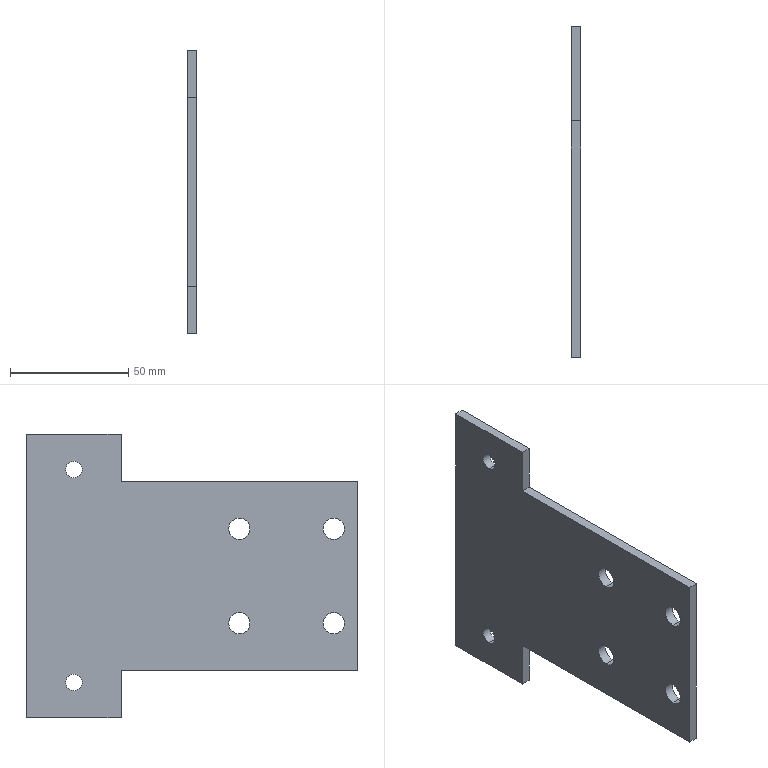Part | SolidWorks | features BaseBody 1 | 1 solid | 22 faces | box 4 x 140 x 120 mm | volume 49874 mm3 | cylinder 12 | plane 10 | commonest cylinder face diameters 9 x8 7 x4
STEP:
#1=CARTESIAN_POINT('',(0.,-90.,-15.5));
#2=VERTEX_POINT('',#1);
#3=CARTESIAN_POINT('',(0.,-90.,-24.5));
#4=VERTEX_POINT('',#3);
#5=CARTESIAN_POINT('',(0.,-90.,-20.));
#6=DIRECTION('',(1.,0.,0.));
#7=DIRECTION('',(0.,0.,1.));
#8=AXIS2_PLACEMENT_3D('',#5,#6,#7);
#9=CIRCLE('',#8,4.5);
#10=EDGE_CURVE('',#2,#4,#9,.T.);
#11=ORIENTED_EDGE('',*,*,#10,.F.);
#12=CARTESIAN_POINT('',(4.,-90.,-15.5));
#13=VERTEX_POINT('',#12);
#14=CARTESIAN_POINT('',(0.,-90.,-15.5));
#15=DIRECTION('',(1.,0.,0.));
#16=VECTOR('',#15,1000.);
#17=LINE('',#14,#16);
#18=EDGE_CURVE('',#2,#13,#17,.T.);
#19=ORIENTED_EDGE('',*,*,#18,.T.);
#20=CARTESIAN_POINT('',(4.,-90.,-24.5));
#21=VERTEX_POINT('',#20);
#22=CARTESIAN_POINT('',(4.,-90.,-20.));
#23=DIRECTION('',(1.,0.,0.));
#24=DIRECTION('',(0.,0.,1.));
#25=AXIS2_PLACEMENT_3D('',#22,#23,#24);
#26=CIRCLE('',#25,4.5);
#27=EDGE_CURVE('',#13,#21,#26,.T.);
#28=ORIENTED_EDGE('',*,*,#27,.T.);
#29=CARTESIAN_POINT('',(0.,-90.,-24.5));
#30=DIRECTION('',(1.,0.,0.));
#31=VECTOR('',#30,1000.);
#32=LINE('',#29,#31);
#33=EDGE_CURVE('',#4,#21,#32,.T.);
#34=ORIENTED_EDGE('',*,*,#33,.F.);
#35=EDGE_LOOP('',(#11,#19,#28,#34));
#36=FACE_OUTER_BOUND('',#35,.T.);
#37=CARTESIAN_POINT('',(0.,-90.,-20.));
#38=DIRECTION('',(1.,0.,0.));
#39=DIRECTION('',(0.,0.,-1.));
#40=AXIS2_PLACEMENT_3D('',#37,#38,#39);
#41=CYLINDRICAL_SURFACE('',#40,4.5);
#42=ADVANCED_FACE('',(#36),#41,.F.);
#43=CARTESIAN_POINT('',(0.,-50.,-15.5));
#44=VERTEX_POINT('',#43);
#45=CARTESIAN_POINT('',(0.,-50.,-24.5));
#46=VERTEX_POINT('',#45);
#47=CARTESIAN_POINT('',(0.,-50.,-20.));
#48=DIRECTION('',(1.,0.,0.));
#49=DIRECTION('',(0.,0.,1.));
#50=AXIS2_PLACEMENT_3D('',#47,#48,#49);
#51=CIRCLE('',#50,4.5);
#52=EDGE_CURVE('',#44,#46,#51,.T.);
#53=ORIENTED_EDGE('',*,*,#52,.F.);
#54=CARTESIAN_POINT('',(4.,-50.,-15.5));
#55=VERTEX_POINT('',#54);
#56=CARTESIAN_POINT('',(0.,-50.,-15.5));
#57=DIRECTION('',(1.,0.,0.));
#58=VECTOR('',#57,1000.);
#59=LINE('',#56,#58);
#60=EDGE_CURVE('',#44,#55,#59,.T.);
#61=ORIENTED_EDGE('',*,*,#60,.T.);
#62=CARTESIAN_POINT('',(4.,-50.,-24.5));
#63=VERTEX_POINT('',#62);
#64=CARTESIAN_POINT('',(4.,-50.,-20.));
#65=DIRECTION('',(1.,0.,0.));
#66=DIRECTION('',(0.,0.,1.));
#67=AXIS2_PLACEMENT_3D('',#64,#65,#66);
#68=CIRCLE('',#67,4.5);
#69=EDGE_CURVE('',#55,#63,#68,.T.);
#70=ORIENTED_EDGE('',*,*,#69,.T.);
#71=CARTESIAN_POINT('',(0.,-50.,-24.5));
#72=DIRECTION('',(1.,0.,0.));
#73=VECTOR('',#72,1000.);
#74=LINE('',#71,#73);
#75=EDGE_CURVE('',#46,#63,#74,.T.);
#76=ORIENTED_EDGE('',*,*,#75,.F.);
#77=EDGE_LOOP('',(#53,#61,#70,#76));
#78=FACE_OUTER_BOUND('',#77,.T.);
#79=CARTESIAN_POINT('',(0.,-50.,-20.));
#80=DIRECTION('',(1.,0.,0.));
#81=DIRECTION('',(0.,0.,-1.));
#82=AXIS2_PLACEMENT_3D('',#79,#80,#81);
#83=CYLINDRICAL_SURFACE('',#82,4.5);
#84=ADVANCED_FACE('',(#78),#83,.F.);
#85=CARTESIAN_POINT('',(0.,-50.,24.5));
#86=VERTEX_POINT('',#85);
#87=CARTESIAN_POINT('',(0.,-50.,15.5));
#88=VERTEX_POINT('',#87);
#89=CARTESIAN_POINT('',(0.,-50.,20.));
#90=DIRECTION('',(1.,0.,0.));
#91=DIRECTION('',(0.,0.,-1.));
#92=AXIS2_PLACEMENT_3D('',#89,#90,#91);
#93=CIRCLE('',#92,4.5);
#94=EDGE_CURVE('',#86,#88,#93,.T.);
#95=ORIENTED_EDGE('',*,*,#94,.F.);
#96=CARTESIAN_POINT('',(4.,-50.,24.5));
#97=VERTEX_POINT('',#96);
#98=CARTESIAN_POINT('',(0.,-50.,24.5));
#99=DIRECTION('',(1.,0.,0.));
#100=VECTOR('',#99,1000.);
#101=LINE('',#98,#100);
#102=EDGE_CURVE('',#86,#97,#101,.T.);
#103=ORIENTED_EDGE('',*,*,#102,.T.);
#104=CARTESIAN_POINT('',(4.,-50.,15.5));
#105=VERTEX_POINT('',#104);
#106=CARTESIAN_POINT('',(4.,-50.,20.));
#107=DIRECTION('',(1.,0.,0.));
#108=DIRECTION('',(0.,0.,-1.));
#109=AXIS2_PLACEMENT_3D('',#106,#107,#108);
#110=CIRCLE('',#109,4.5);
#111=EDGE_CURVE('',#97,#105,#110,.T.);
#112=ORIENTED_EDGE('',*,*,#111,.T.);
#113=CARTESIAN_POINT('',(0.,-50.,15.5));
#114=DIRECTION('',(1.,0.,0.));
#115=VECTOR('',#114,1000.);
#116=LINE('',#113,#115);
#117=EDGE_CURVE('',#88,#105,#116,.T.);
#118=ORIENTED_EDGE('',*,*,#117,.F.);
#119=EDGE_LOOP('',(#95,#103,#112,#118));
#120=FACE_OUTER_BOUND('',#119,.T.);
#121=CARTESIAN_POINT('',(0.,-50.,20.));
#122=DIRECTION('',(1.,0.,0.));
#123=DIRECTION('',(0.,0.,-1.));
#124=AXIS2_PLACEMENT_3D('',#121,#122,#123);
#125=CYLINDRICAL_SURFACE('',#124,4.5);
#126=ADVANCED_FACE('',(#120),#125,.F.);
#127=CARTESIAN_POINT('',(0.,20.,-41.5));
#128=VERTEX_POINT('',#127);
#129=CARTESIAN_POINT('',(0.,20.,-48.5));
#130=VERTEX_POINT('',#129);
#131=CARTESIAN_POINT('',(0.,20.,-45.));
#132=DIRECTION('',(1.,0.,0.));
#133=DIRECTION('',(0.,0.,-1.));
#134=AXIS2_PLACEMENT_3D('',#131,#132,#133);
#135=CIRCLE('',#134,3.5);
#136=EDGE_CURVE('',#128,#130,#135,.T.);
#137=ORIENTED_EDGE('',*,*,#136,.F.);
#138=CARTESIAN_POINT('',(4.,20.,-41.5));
#139=VERTEX_POINT('',#138);
#140=CARTESIAN_POINT('',(0.,20.,-41.5));
#141=DIRECTION('',(1.,0.,0.));
#142=VECTOR('',#141,1000.);
#143=LINE('',#140,#142);
#144=EDGE_CURVE('',#128,#139,#143,.T.);
#145=ORIENTED_EDGE('',*,*,#144,.T.);
#146=CARTESIAN_POINT('',(4.,20.,-48.5));
#147=VERTEX_POINT('',#146);
#148=CARTESIAN_POINT('',(4.,20.,-45.));
#149=DIRECTION('',(1.,0.,0.));
#150=DIRECTION('',(0.,0.,-1.));
#151=AXIS2_PLACEMENT_3D('',#148,#149,#150);
#152=CIRCLE('',#151,3.5);
#153=EDGE_CURVE('',#139,#147,#152,.T.);
#154=ORIENTED_EDGE('',*,*,#153,.T.);
#155=CARTESIAN_POINT('',(0.,20.,-48.5));
#156=DIRECTION('',(1.,0.,0.));
#157=VECTOR('',#156,1000.);
#158=LINE('',#155,#157);
#159=EDGE_CURVE('',#130,#147,#158,.T.);
#160=ORIENTED_EDGE('',*,*,#159,.F.);
#161=EDGE_LOOP('',(#137,#145,#154,#160));
#162=FACE_OUTER_BOUND('',#161,.T.);
#163=CARTESIAN_POINT('',(0.,20.,-45.));
#164=DIRECTION('',(1.,0.,0.));
#165=DIRECTION('',(0.,0.,-1.));
#166=AXIS2_PLACEMENT_3D('',#163,#164,#165);
#167=CYLINDRICAL_SURFACE('',#166,3.5);
#168=ADVANCED_FACE('',(#162),#167,.F.);
#169=CARTESIAN_POINT('',(0.,20.,48.5));
#170=VERTEX_POINT('',#169);
#171=CARTESIAN_POINT('',(0.,20.,41.5));
#172=VERTEX_POINT('',#171);
#173=CARTESIAN_POINT('',(0.,20.,45.));
#174=DIRECTION('',(1.,0.,0.));
#175=DIRECTION('',(0.,0.,1.));
#176=AXIS2_PLACEMENT_3D('',#173,#174,#175);
#177=CIRCLE('',#176,3.5);
#178=EDGE_CURVE('',#170,#172,#177,.T.);
#179=ORIENTED_EDGE('',*,*,#178,.F.);
#180=CARTESIAN_POINT('',(4.,20.,48.5));
#181=VERTEX_POINT('',#180);
#182=CARTESIAN_POINT('',(0.,20.,48.5));
#183=DIRECTION('',(1.,0.,0.));
#184=VECTOR('',#183,1000.);
#185=LINE('',#182,#184);
#186=EDGE_CURVE('',#170,#181,#185,.T.);
#187=ORIENTED_EDGE('',*,*,#186,.T.);
#188=CARTESIAN_POINT('',(4.,20.,41.5));
#189=VERTEX_POINT('',#188);
#190=CARTESIAN_POINT('',(4.,20.,45.));
#191=DIRECTION('',(1.,0.,0.));
#192=DIRECTION('',(0.,0.,1.));
#193=AXIS2_PLACEMENT_3D('',#190,#191,#192);
#194=CIRCLE('',#193,3.5);
#195=EDGE_CURVE('',#181,#189,#194,.T.);
#196=ORIENTED_EDGE('',*,*,#195,.T.);
#197=CARTESIAN_POINT('',(0.,20.,41.5));
#198=DIRECTION('',(1.,0.,0.));
#199=VECTOR('',#198,1000.);
#200=LINE('',#197,#199);
#201=EDGE_CURVE('',#172,#189,#200,.T.);
#202=ORIENTED_EDGE('',*,*,#201,.F.);
#203=EDGE_LOOP('',(#179,#187,#196,#202));
#204=FACE_OUTER_BOUND('',#203,.T.);
#205=CARTESIAN_POINT('',(0.,20.,45.));
#206=DIRECTION('',(1.,0.,0.));
#207=DIRECTION('',(0.,0.,-1.));
#208=AXIS2_PLACEMENT_3D('',#205,#206,#207);
#209=CYLINDRICAL_SURFACE('',#208,3.5);
#210=ADVANCED_FACE('',(#204),#209,.F.);
#211=CARTESIAN_POINT('',(0.,-90.,24.5));
#212=VERTEX_POINT('',#211);
#213=CARTESIAN_POINT('',(0.,-90.,15.5));
#214=VERTEX_POINT('',#213);
#215=CARTESIAN_POINT('',(0.,-90.,20.));
#216=DIRECTION('',(1.,0.,0.));
#217=DIRECTION('',(0.,0.,-1.));
#218=AXIS2_PLACEMENT_3D('',#215,#216,#217);
#219=CIRCLE('',#218,4.5);
#220=EDGE_CURVE('',#212,#214,#219,.T.);
#221=ORIENTED_EDGE('',*,*,#220,.F.);
#222=CARTESIAN_POINT('',(4.,-90.,24.5));
#223=VERTEX_POINT('',#222);
#224=CARTESIAN_POINT('',(0.,-90.,24.5));
#225=DIRECTION('',(1.,0.,0.));
#226=VECTOR('',#225,1000.);
#227=LINE('',#224,#226);
#228=EDGE_CURVE('',#212,#223,#227,.T.);
#229=ORIENTED_EDGE('',*,*,#228,.T.);
#230=CARTESIAN_POINT('',(4.,-90.,15.5));
#231=VERTEX_POINT('',#230);
#232=CARTESIAN_POINT('',(4.,-90.,20.));
#233=DIRECTION('',(1.,0.,0.));
#234=DIRECTION('',(0.,0.,-1.));
#235=AXIS2_PLACEMENT_3D('',#232,#233,#234);
#236=CIRCLE('',#235,4.5);
#237=EDGE_CURVE('',#223,#231,#236,.T.);
#238=ORIENTED_EDGE('',*,*,#237,.T.);
#239=CARTESIAN_POINT('',(0.,-90.,15.5));
#240=DIRECTION('',(1.,0.,0.));
#241=VECTOR('',#240,1000.);
#242=LINE('',#239,#241);
#243=EDGE_CURVE('',#214,#231,#242,.T.);
#244=ORIENTED_EDGE('',*,*,#243,.F.);
#245=EDGE_LOOP('',(#221,#229,#238,#244));
#246=FACE_OUTER_BOUND('',#245,.T.);
#247=CARTESIAN_POINT('',(0.,-90.,20.));
#248=DIRECTION('',(1.,0.,0.));
#249=DIRECTION('',(0.,0.,-1.));
#250=AXIS2_PLACEMENT_3D('',#247,#248,#249);
#251=CYLINDRICAL_SURFACE('',#250,4.5);
#252=ADVANCED_FACE('',(#246),#251,.F.);
#253=CARTESIAN_POINT('',(0.,-90.,20.));
#254=DIRECTION('',(1.,0.,0.));
#255=DIRECTION('',(0.,0.,-1.));
#256=AXIS2_PLACEMENT_3D('',#253,#254,#255);
#257=CIRCLE('',#256,4.5);
#258=EDGE_CURVE('',#214,#212,#257,.T.);
#259=ORIENTED_EDGE('',*,*,#258,.T.);
#260=ORIENTED_EDGE('',*,*,#220,.T.);
#261=EDGE_LOOP('',(#259,#260));
#262=FACE_BOUND('',#261,.T.);
#263=CARTESIAN_POINT('',(0.,20.,45.));
#264=DIRECTION('',(1.,0.,0.));
#265=DIRECTION('',(0.,0.,1.));
#266=AXIS2_PLACEMENT_3D('',#263,#264,#265);
#267=CIRCLE('',#266,3.5);
#268=EDGE_CURVE('',#172,#170,#267,.T.);
#269=ORIENTED_EDGE('',*,*,#268,.T.);
#270=ORIENTED_EDGE('',*,*,#178,.T.);
#271=EDGE_LOOP('',(#269,#270));
#272=FACE_BOUND('',#271,.T.);
#273=CARTESIAN_POINT('',(0.,20.,-45.));
#274=DIRECTION('',(1.,0.,0.));
#275=DIRECTION('',(0.,0.,-1.));
#276=AXIS2_PLACEMENT_3D('',#273,#274,#275);
#277=CIRCLE('',#276,3.5);
#278=EDGE_CURVE('',#130,#128,#277,.T.);
#279=ORIENTED_EDGE('',*,*,#278,.T.);
#280=ORIENTED_EDGE('',*,*,#136,.T.);
#281=EDGE_LOOP('',(#279,#280));
#282=FACE_BOUND('',#281,.T.);
#283=CARTESIAN_POINT('',(0.,-50.,20.));
#284=DIRECTION('',(1.,0.,0.));
#285=DIRECTION('',(0.,0.,-1.));
#286=AXIS2_PLACEMENT_3D('',#283,#284,#285);
#287=CIRCLE('',#286,4.5);
#288=EDGE_CURVE('',#88,#86,#287,.T.);
#289=ORIENTED_EDGE('',*,*,#288,.T.);
#290=ORIENTED_EDGE('',*,*,#94,.T.);
#291=EDGE_LOOP('',(#289,#290));
#292=FACE_BOUND('',#291,.T.);
#293=CARTESIAN_POINT('',(0.,-50.,-20.));
#294=DIRECTION('',(1.,0.,0.));
#295=DIRECTION('',(0.,0.,1.));
#296=AXIS2_PLACEMENT_3D('',#293,#294,#295);
#297=CIRCLE('',#296,4.5);
#298=EDGE_CURVE('',#46,#44,#297,.T.);
#299=ORIENTED_EDGE('',*,*,#298,.T.);
#300=ORIENTED_EDGE('',*,*,#52,.T.);
#301=EDGE_LOOP('',(#299,#300));
#302=FACE_BOUND('',#301,.T.);
#303=CARTESIAN_POINT('',(0.,-90.,-20.));
#304=DIRECTION('',(1.,0.,0.));
#305=DIRECTION('',(0.,0.,1.));
#306=AXIS2_PLACEMENT_3D('',#303,#304,#305);
#307=CIRCLE('',#306,4.5);
#308=EDGE_CURVE('',#4,#2,#307,.T.);
#309=ORIENTED_EDGE('',*,*,#308,.T.);
#310=ORIENTED_EDGE('',*,*,#10,.T.);
#311=EDGE_LOOP('',(#309,#310));
#312=FACE_BOUND('',#311,.T.);
#313=CARTESIAN_POINT('',(0.,0.,-60.));
#314=VERTEX_POINT('',#313);
#315=CARTESIAN_POINT('',(0.,40.,-60.));
#316=VERTEX_POINT('',#315);
#317=CARTESIAN_POINT('',(0.,0.,-60.));
#318=DIRECTION('',(0.,1.,0.));
#319=VECTOR('',#318,1000.);
#320=LINE('',#317,#319);
#321=EDGE_CURVE('',#314,#316,#320,.T.);
#322=ORIENTED_EDGE('',*,*,#321,.F.);
#323=CARTESIAN_POINT('',(0.,0.,-40.));
#324=VERTEX_POINT('',#323);
#325=CARTESIAN_POINT('',(0.,0.,-60.));
#326=DIRECTION('',(0.,0.,-1.));
#327=VECTOR('',#326,1000.);
#328=LINE('',#325,#327);
#329=EDGE_CURVE('',#324,#314,#328,.T.);
#330=ORIENTED_EDGE('',*,*,#329,.F.);
#331=CARTESIAN_POINT('',(0.,-100.,-40.));
#332=VERTEX_POINT('',#331);
#333=CARTESIAN_POINT('',(0.,0.,-40.));
#334=DIRECTION('',(0.,1.,0.));
#335=VECTOR('',#334,1000.);
#336=LINE('',#333,#335);
#337=EDGE_CURVE('',#332,#324,#336,.T.);
#338=ORIENTED_EDGE('',*,*,#337,.F.);
#339=CARTESIAN_POINT('',(0.,-100.,40.));
#340=VERTEX_POINT('',#339);
#341=CARTESIAN_POINT('',(0.,-100.,40.));
#342=DIRECTION('',(0.,0.,-1.));
#343=VECTOR('',#342,1000.);
#344=LINE('',#341,#343);
#345=EDGE_CURVE('',#340,#332,#344,.T.);
#346=ORIENTED_EDGE('',*,*,#345,.F.);
#347=CARTESIAN_POINT('',(0.,0.,40.));
#348=VERTEX_POINT('',#347);
#349=CARTESIAN_POINT('',(0.,0.,40.));
#350=DIRECTION('',(0.,-1.,0.));
#351=VECTOR('',#350,1000.);
#352=LINE('',#349,#351);
#353=EDGE_CURVE('',#348,#340,#352,.T.);
#354=ORIENTED_EDGE('',*,*,#353,.F.);
#355=CARTESIAN_POINT('',(0.,0.,60.));
#356=VERTEX_POINT('',#355);
#357=CARTESIAN_POINT('',(0.,0.,40.));
#358=DIRECTION('',(0.,0.,-1.));
#359=VECTOR('',#358,1000.);
#360=LINE('',#357,#359);
#361=EDGE_CURVE('',#356,#348,#360,.T.);
#362=ORIENTED_EDGE('',*,*,#361,.F.);
#363=CARTESIAN_POINT('',(0.,40.,60.));
#364=VERTEX_POINT('',#363);
#365=CARTESIAN_POINT('',(0.,0.,60.));
#366=DIRECTION('',(0.,-1.,0.));
#367=VECTOR('',#366,1000.);
#368=LINE('',#365,#367);
#369=EDGE_CURVE('',#364,#356,#368,.T.);
#370=ORIENTED_EDGE('',*,*,#369,.F.);
#371=CARTESIAN_POINT('',(0.,40.,-60.));
#372=DIRECTION('',(0.,0.,1.));
#373=VECTOR('',#372,1000.);
#374=LINE('',#371,#373);
#375=EDGE_CURVE('',#316,#364,#374,.T.);
#376=ORIENTED_EDGE('',*,*,#375,.F.);
#377=EDGE_LOOP('',(#322,#330,#338,#346,#354,#362,#370,#376));
#378=FACE_OUTER_BOUND('',#377,.T.);
#379=CARTESIAN_POINT('',(0.,0.,0.));
#380=DIRECTION('',(1.,0.,0.));
#381=DIRECTION('',(0.,1.,0.));
#382=AXIS2_PLACEMENT_3D('',#379,#380,#381);
#383=PLANE('',#382);
#384=ADVANCED_FACE('',(#262,#272,#282,#292,#302,#312,#378),#383,.F.);
#385=CARTESIAN_POINT('',(4.,-90.,20.));
#386=DIRECTION('',(1.,0.,0.));
#387=DIRECTION('',(0.,0.,-1.));
#388=AXIS2_PLACEMENT_3D('',#385,#386,#387);
#389=CIRCLE('',#388,4.5);
#390=EDGE_CURVE('',#231,#223,#389,.T.);
#391=ORIENTED_EDGE('',*,*,#390,.F.);
#392=ORIENTED_EDGE('',*,*,#237,.F.);
#393=EDGE_LOOP('',(#391,#392));
#394=FACE_BOUND('',#393,.T.);
#395=CARTESIAN_POINT('',(4.,20.,45.));
#396=DIRECTION('',(1.,0.,0.));
#397=DIRECTION('',(0.,0.,1.));
#398=AXIS2_PLACEMENT_3D('',#395,#396,#397);
#399=CIRCLE('',#398,3.5);
#400=EDGE_CURVE('',#189,#181,#399,.T.);
#401=ORIENTED_EDGE('',*,*,#400,.F.);
#402=ORIENTED_EDGE('',*,*,#195,.F.);
#403=EDGE_LOOP('',(#401,#402));
#404=FACE_BOUND('',#403,.T.);
#405=CARTESIAN_POINT('',(4.,20.,-45.));
#406=DIRECTION('',(1.,0.,0.));
#407=DIRECTION('',(0.,0.,-1.));
#408=AXIS2_PLACEMENT_3D('',#405,#406,#407);
#409=CIRCLE('',#408,3.5);
#410=EDGE_CURVE('',#147,#139,#409,.T.);
#411=ORIENTED_EDGE('',*,*,#410,.F.);
#412=ORIENTED_EDGE('',*,*,#153,.F.);
#413=EDGE_LOOP('',(#411,#412));
#414=FACE_BOUND('',#413,.T.);
#415=CARTESIAN_POINT('',(4.,-50.,20.));
#416=DIRECTION('',(1.,0.,0.));
#417=DIRECTION('',(0.,0.,-1.));
#418=AXIS2_PLACEMENT_3D('',#415,#416,#417);
#419=CIRCLE('',#418,4.5);
#420=EDGE_CURVE('',#105,#97,#419,.T.);
#421=ORIENTED_EDGE('',*,*,#420,.F.);
#422=ORIENTED_EDGE('',*,*,#111,.F.);
#423=EDGE_LOOP('',(#421,#422));
#424=FACE_BOUND('',#423,.T.);
#425=CARTESIAN_POINT('',(4.,-50.,-20.));
#426=DIRECTION('',(1.,0.,0.));
#427=DIRECTION('',(0.,0.,1.));
#428=AXIS2_PLACEMENT_3D('',#425,#426,#427);
#429=CIRCLE('',#428,4.5);
#430=EDGE_CURVE('',#63,#55,#429,.T.);
#431=ORIENTED_EDGE('',*,*,#430,.F.);
#432=ORIENTED_EDGE('',*,*,#69,.F.);
#433=EDGE_LOOP('',(#431,#432));
#434=FACE_BOUND('',#433,.T.);
#435=CARTESIAN_POINT('',(4.,-90.,-20.));
#436=DIRECTION('',(1.,0.,0.));
#437=DIRECTION('',(0.,0.,1.));
#438=AXIS2_PLACEMENT_3D('',#435,#436,#437);
#439=CIRCLE('',#438,4.5);
#440=EDGE_CURVE('',#21,#13,#439,.T.);
#441=ORIENTED_EDGE('',*,*,#440,.F.);
#442=ORIENTED_EDGE('',*,*,#27,.F.);
#443=EDGE_LOOP('',(#441,#442));
#444=FACE_BOUND('',#443,.T.);
#445=CARTESIAN_POINT('',(4.,0.,-60.));
#446=VERTEX_POINT('',#445);
#447=CARTESIAN_POINT('',(4.,40.,-60.));
#448=VERTEX_POINT('',#447);
#449=CARTESIAN_POINT('',(4.,0.,-60.));
#450=DIRECTION('',(0.,1.,0.));
#451=VECTOR('',#450,1000.);
#452=LINE('',#449,#451);
#453=EDGE_CURVE('',#446,#448,#452,.T.);
#454=ORIENTED_EDGE('',*,*,#453,.T.);
#455=CARTESIAN_POINT('',(4.,40.,60.));
#456=VERTEX_POINT('',#455);
#457=CARTESIAN_POINT('',(4.,40.,-60.));
#458=DIRECTION('',(0.,0.,1.));
#459=VECTOR('',#458,1000.);
#460=LINE('',#457,#459);
#461=EDGE_CURVE('',#448,#456,#460,.T.);
#462=ORIENTED_EDGE('',*,*,#461,.T.);
#463=CARTESIAN_POINT('',(4.,0.,60.));
#464=VERTEX_POINT('',#463);
#465=CARTESIAN_POINT('',(4.,0.,60.));
#466=DIRECTION('',(0.,-1.,0.));
#467=VECTOR('',#466,1000.);
#468=LINE('',#465,#467);
#469=EDGE_CURVE('',#456,#464,#468,.T.);
#470=ORIENTED_EDGE('',*,*,#469,.T.);
#471=CARTESIAN_POINT('',(4.,0.,40.));
#472=VERTEX_POINT('',#471);
#473=CARTESIAN_POINT('',(4.,0.,40.));
#474=DIRECTION('',(0.,0.,-1.));
#475=VECTOR('',#474,1000.);
#476=LINE('',#473,#475);
#477=EDGE_CURVE('',#464,#472,#476,.T.);
#478=ORIENTED_EDGE('',*,*,#477,.T.);
#479=CARTESIAN_POINT('',(4.,-100.,40.));
#480=VERTEX_POINT('',#479);
#481=CARTESIAN_POINT('',(4.,0.,40.));
#482=DIRECTION('',(0.,-1.,0.));
#483=VECTOR('',#482,1000.);
#484=LINE('',#481,#483);
#485=EDGE_CURVE('',#472,#480,#484,.T.);
#486=ORIENTED_EDGE('',*,*,#485,.T.);
#487=CARTESIAN_POINT('',(4.,-100.,-40.));
#488=VERTEX_POINT('',#487);
#489=CARTESIAN_POINT('',(4.,-100.,40.));
#490=DIRECTION('',(0.,0.,-1.));
#491=VECTOR('',#490,1000.);
#492=LINE('',#489,#491);
#493=EDGE_CURVE('',#480,#488,#492,.T.);
#494=ORIENTED_EDGE('',*,*,#493,.T.);
#495=CARTESIAN_POINT('',(4.,0.,-40.));
#496=VERTEX_POINT('',#495);
#497=CARTESIAN_POINT('',(4.,0.,-40.));
#498=DIRECTION('',(0.,1.,0.));
#499=VECTOR('',#498,1000.);
#500=LINE('',#497,#499);
#501=EDGE_CURVE('',#488,#496,#500,.T.);
#502=ORIENTED_EDGE('',*,*,#501,.T.);
#503=CARTESIAN_POINT('',(4.,0.,-60.));
#504=DIRECTION('',(0.,0.,-1.));
#505=VECTOR('',#504,1000.);
#506=LINE('',#503,#505);
#507=EDGE_CURVE('',#496,#446,#506,.T.);
#508=ORIENTED_EDGE('',*,*,#507,.T.);
#509=EDGE_LOOP('',(#454,#462,#470,#478,#486,#494,#502,#508));
#510=FACE_OUTER_BOUND('',#509,.T.);
#511=CARTESIAN_POINT('',(4.,0.,0.));
#512=DIRECTION('',(1.,0.,0.));
#513=DIRECTION('',(0.,1.,0.));
#514=AXIS2_PLACEMENT_3D('',#511,#512,#513);
#515=PLANE('',#514);
#516=ADVANCED_FACE('',(#394,#404,#414,#424,#434,#444,#510),#515,.T.);
#517=ORIENTED_EDGE('',*,*,#329,.T.);
#518=CARTESIAN_POINT('',(4.,0.,-60.));
#519=DIRECTION('',(-1.,0.,0.));
#520=VECTOR('',#519,1000.);
#521=LINE('',#518,#520);
#522=EDGE_CURVE('',#446,#314,#521,.T.);
#523=ORIENTED_EDGE('',*,*,#522,.F.);
#524=ORIENTED_EDGE('',*,*,#507,.F.);
#525=CARTESIAN_POINT('',(4.,0.,-40.));
#526=DIRECTION('',(-1.,0.,0.));
#527=VECTOR('',#526,1000.);
#528=LINE('',#525,#527);
#529=EDGE_CURVE('',#496,#324,#528,.T.);
#530=ORIENTED_EDGE('',*,*,#529,.T.);
#531=EDGE_LOOP('',(#517,#523,#524,#530));
#532=FACE_OUTER_BOUND('',#531,.T.);
#533=CARTESIAN_POINT('',(4.,0.,-60.));
#534=DIRECTION('',(0.,1.,0.));
#535=DIRECTION('',(0.,0.,-1.));
#536=AXIS2_PLACEMENT_3D('',#533,#534,#535);
#537=PLANE('',#536);
#538=ADVANCED_FACE('',(#532),#537,.F.);
#539=ORIENTED_EDGE('',*,*,#337,.T.);
#540=ORIENTED_EDGE('',*,*,#529,.F.);
#541=ORIENTED_EDGE('',*,*,#501,.F.);
#542=CARTESIAN_POINT('',(4.,-100.,-40.));
#543=DIRECTION('',(-1.,0.,0.));
#544=VECTOR('',#543,1000.);
#545=LINE('',#542,#544);
#546=EDGE_CURVE('',#488,#332,#545,.T.);
#547=ORIENTED_EDGE('',*,*,#546,.T.);
#548=EDGE_LOOP('',(#539,#540,#541,#547));
#549=FACE_OUTER_BOUND('',#548,.T.);
#550=CARTESIAN_POINT('',(4.,0.,-40.));
#551=DIRECTION('',(0.,0.,1.));
#552=DIRECTION('',(0.,-1.,0.));
#553=AXIS2_PLACEMENT_3D('',#550,#551,#552);
#554=PLANE('',#553);
#555=ADVANCED_FACE('',(#549),#554,.F.);
#556=ORIENTED_EDGE('',*,*,#345,.T.);
#557=ORIENTED_EDGE('',*,*,#546,.F.);
#558=ORIENTED_EDGE('',*,*,#493,.F.);
#559=CARTESIAN_POINT('',(4.,-100.,40.));
#560=DIRECTION('',(-1.,0.,0.));
#561=VECTOR('',#560,1000.);
#562=LINE('',#559,#561);
#563=EDGE_CURVE('',#480,#340,#562,.T.);
#564=ORIENTED_EDGE('',*,*,#563,.T.);
#565=EDGE_LOOP('',(#556,#557,#558,#564));
#566=FACE_OUTER_BOUND('',#565,.T.);
#567=CARTESIAN_POINT('',(4.,-100.,40.));
#568=DIRECTION('',(0.,1.,0.));
#569=DIRECTION('',(1.,0.,0.));
#570=AXIS2_PLACEMENT_3D('',#567,#568,#569);
#571=PLANE('',#570);
#572=ADVANCED_FACE('',(#566),#571,.F.);
#573=ORIENTED_EDGE('',*,*,#353,.T.);
#574=ORIENTED_EDGE('',*,*,#563,.F.);
#575=ORIENTED_EDGE('',*,*,#485,.F.);
#576=CARTESIAN_POINT('',(4.,0.,40.));
#577=DIRECTION('',(-1.,0.,0.));
#578=VECTOR('',#577,1000.);
#579=LINE('',#576,#578);
#580=EDGE_CURVE('',#472,#348,#579,.T.);
#581=ORIENTED_EDGE('',*,*,#580,.T.);
#582=EDGE_LOOP('',(#573,#574,#575,#581));
#583=FACE_OUTER_BOUND('',#582,.T.);
#584=CARTESIAN_POINT('',(4.,0.,40.));
#585=DIRECTION('',(0.,0.,-1.));
#586=DIRECTION('',(0.,-1.,0.));
#587=AXIS2_PLACEMENT_3D('',#584,#585,#586);
#588=PLANE('',#587);
#589=ADVANCED_FACE('',(#583),#588,.F.);
#590=ORIENTED_EDGE('',*,*,#361,.T.);
#591=ORIENTED_EDGE('',*,*,#580,.F.);
#592=ORIENTED_EDGE('',*,*,#477,.F.);
#593=CARTESIAN_POINT('',(4.,0.,60.));
#594=DIRECTION('',(-1.,0.,0.));
#595=VECTOR('',#594,1000.);
#596=LINE('',#593,#595);
#597=EDGE_CURVE('',#464,#356,#596,.T.);
#598=ORIENTED_EDGE('',*,*,#597,.T.);
#599=EDGE_LOOP('',(#590,#591,#592,#598));
#600=FACE_OUTER_BOUND('',#599,.T.);
#601=CARTESIAN_POINT('',(4.,0.,40.));
#602=DIRECTION('',(0.,1.,0.));
#603=DIRECTION('',(0.,0.,-1.));
#604=AXIS2_PLACEMENT_3D('',#601,#602,#603);
#605=PLANE('',#604);
#606=ADVANCED_FACE('',(#600),#605,.F.);
#607=ORIENTED_EDGE('',*,*,#369,.T.);
#608=ORIENTED_EDGE('',*,*,#597,.F.);
#609=ORIENTED_EDGE('',*,*,#469,.F.);
#610=CARTESIAN_POINT('',(4.,40.,60.));
#611=DIRECTION('',(-1.,0.,0.));
#612=VECTOR('',#611,1000.);
#613=LINE('',#610,#612);
#614=EDGE_CURVE('',#456,#364,#613,.T.);
#615=ORIENTED_EDGE('',*,*,#614,.T.);
#616=EDGE_LOOP('',(#607,#608,#609,#615));
#617=FACE_OUTER_BOUND('',#616,.T.);
#618=CARTESIAN_POINT('',(4.,0.,60.));
#619=DIRECTION('',(0.,0.,-1.));
#620=DIRECTION('',(0.,-1.,0.));
#621=AXIS2_PLACEMENT_3D('',#618,#619,#620);
#622=PLANE('',#621);
#623=ADVANCED_FACE('',(#617),#622,.F.);
#624=ORIENTED_EDGE('',*,*,#375,.T.);
#625=ORIENTED_EDGE('',*,*,#614,.F.);
#626=ORIENTED_EDGE('',*,*,#461,.F.);
#627=CARTESIAN_POINT('',(4.,40.,-60.));
#628=DIRECTION('',(-1.,0.,0.));
#629=VECTOR('',#628,1000.);
#630=LINE('',#627,#629);
#631=EDGE_CURVE('',#448,#316,#630,.T.);
#632=ORIENTED_EDGE('',*,*,#631,.T.);
#633=EDGE_LOOP('',(#624,#625,#626,#632));
#634=FACE_OUTER_BOUND('',#633,.T.);
#635=CARTESIAN_POINT('',(4.,40.,-60.));
#636=DIRECTION('',(0.,-1.,0.));
#637=DIRECTION('',(0.,0.,-1.));
#638=AXIS2_PLACEMENT_3D('',#635,#636,#637);
#639=PLANE('',#638);
#640=ADVANCED_FACE('',(#634),#639,.F.);
#641=ORIENTED_EDGE('',*,*,#321,.T.);
#642=ORIENTED_EDGE('',*,*,#631,.F.);
#643=ORIENTED_EDGE('',*,*,#453,.F.);
#644=ORIENTED_EDGE('',*,*,#522,.T.);
#645=EDGE_LOOP('',(#641,#642,#643,#644));
#646=FACE_OUTER_BOUND('',#645,.T.);
#647=CARTESIAN_POINT('',(4.,0.,-60.));
#648=DIRECTION('',(0.,0.,1.));
#649=DIRECTION('',(1.,0.,0.));
#650=AXIS2_PLACEMENT_3D('',#647,#648,#649);
#651=PLANE('',#650);
#652=ADVANCED_FACE('',(#646),#651,.F.);
#653=ORIENTED_EDGE('',*,*,#228,.F.);
#654=ORIENTED_EDGE('',*,*,#258,.F.);
#655=ORIENTED_EDGE('',*,*,#243,.T.);
#656=ORIENTED_EDGE('',*,*,#390,.T.);
#657=EDGE_LOOP('',(#653,#654,#655,#656));
#658=FACE_OUTER_BOUND('',#657,.T.);
#659=CARTESIAN_POINT('',(0.,-90.,20.));
#660=DIRECTION('',(1.,0.,0.));
#661=DIRECTION('',(0.,0.,-1.));
#662=AXIS2_PLACEMENT_3D('',#659,#660,#661);
#663=CYLINDRICAL_SURFACE('',#662,4.5);
#664=ADVANCED_FACE('',(#658),#663,.F.);
#665=ORIENTED_EDGE('',*,*,#186,.F.);
#666=ORIENTED_EDGE('',*,*,#268,.F.);
#667=ORIENTED_EDGE('',*,*,#201,.T.);
#668=ORIENTED_EDGE('',*,*,#400,.T.);
#669=EDGE_LOOP('',(#665,#666,#667,#668));
#670=FACE_OUTER_BOUND('',#669,.T.);
#671=CARTESIAN_POINT('',(0.,20.,45.));
#672=DIRECTION('',(1.,0.,0.));
#673=DIRECTION('',(0.,0.,-1.));
#674=AXIS2_PLACEMENT_3D('',#671,#672,#673);
#675=CYLINDRICAL_SURFACE('',#674,3.5);
#676=ADVANCED_FACE('',(#670),#675,.F.);
#677=ORIENTED_EDGE('',*,*,#144,.F.);
#678=ORIENTED_EDGE('',*,*,#278,.F.);
#679=ORIENTED_EDGE('',*,*,#159,.T.);
#680=ORIENTED_EDGE('',*,*,#410,.T.);
#681=EDGE_LOOP('',(#677,#678,#679,#680));
#682=FACE_OUTER_BOUND('',#681,.T.);
#683=CARTESIAN_POINT('',(0.,20.,-45.));
#684=DIRECTION('',(1.,0.,0.));
#685=DIRECTION('',(0.,0.,-1.));
#686=AXIS2_PLACEMENT_3D('',#683,#684,#685);
#687=CYLINDRICAL_SURFACE('',#686,3.5);
#688=ADVANCED_FACE('',(#682),#687,.F.);
#689=ORIENTED_EDGE('',*,*,#102,.F.);
#690=ORIENTED_EDGE('',*,*,#288,.F.);
#691=ORIENTED_EDGE('',*,*,#117,.T.);
#692=ORIENTED_EDGE('',*,*,#420,.T.);
#693=EDGE_LOOP('',(#689,#690,#691,#692));
#694=FACE_OUTER_BOUND('',#693,.T.);
#695=CARTESIAN_POINT('',(0.,-50.,20.));
#696=DIRECTION('',(1.,0.,0.));
#697=DIRECTION('',(0.,0.,-1.));
#698=AXIS2_PLACEMENT_3D('',#695,#696,#697);
#699=CYLINDRICAL_SURFACE('',#698,4.5);
#700=ADVANCED_FACE('',(#694),#699,.F.);
#701=ORIENTED_EDGE('',*,*,#60,.F.);
#702=ORIENTED_EDGE('',*,*,#298,.F.);
#703=ORIENTED_EDGE('',*,*,#75,.T.);
#704=ORIENTED_EDGE('',*,*,#430,.T.);
#705=EDGE_LOOP('',(#701,#702,#703,#704));
#706=FACE_OUTER_BOUND('',#705,.T.);
#707=CARTESIAN_POINT('',(0.,-50.,-20.));
#708=DIRECTION('',(1.,0.,0.));
#709=DIRECTION('',(0.,0.,-1.));
#710=AXIS2_PLACEMENT_3D('',#707,#708,#709);
#711=CYLINDRICAL_SURFACE('',#710,4.5);
#712=ADVANCED_FACE('',(#706),#711,.F.);
#713=ORIENTED_EDGE('',*,*,#18,.F.);
#714=ORIENTED_EDGE('',*,*,#308,.F.);
#715=ORIENTED_EDGE('',*,*,#33,.T.);
#716=ORIENTED_EDGE('',*,*,#440,.T.);
#717=EDGE_LOOP('',(#713,#714,#715,#716));
#718=FACE_OUTER_BOUND('',#717,.T.);
#719=CARTESIAN_POINT('',(0.,-90.,-20.));
#720=DIRECTION('',(1.,0.,0.));
#721=DIRECTION('',(0.,0.,-1.));
#722=AXIS2_PLACEMENT_3D('',#719,#720,#721);
#723=CYLINDRICAL_SURFACE('',#722,4.5);
#724=ADVANCED_FACE('',(#718),#723,.F.);
#725=CLOSED_SHELL('',(#42,#84,#126,#168,#210,#252,#384,#516,#538,#555,#572,#589,#606,#623,#640,#652,#664,#676,#688,#700,#712,#724));
#726=MANIFOLD_SOLID_BREP('',#725);
#727=CARTESIAN_POINT('',(0.,0.,0.));
#728=DIRECTION('',(0.,0.,1.));
#729=DIRECTION('',(1.,0.,0.));
#730=AXIS2_PLACEMENT_3D('',#727,#728,#729);
#731=(LENGTH_UNIT()NAMED_UNIT(*)SI_UNIT(.MILLI.,.METRE.));
#732=UNCERTAINTY_MEASURE_WITH_UNIT(LENGTH_MEASURE(0.00001),#731,'','');
#733=(NAMED_UNIT(*)PLANE_ANGLE_UNIT()SI_UNIT($,.RADIAN.));
#734=(NAMED_UNIT(*)SI_UNIT($,.STERADIAN.)SOLID_ANGLE_UNIT());
#735=(GEOMETRIC_REPRESENTATION_CONTEXT(3)GLOBAL_UNCERTAINTY_ASSIGNED_CONTEXT((#732))GLOBAL_UNIT_ASSIGNED_CONTEXT((#731,#733,#734))REPRESENTATION_CONTEXT('',''));
#736=ADVANCED_BREP_SHAPE_REPRESENTATION('',(#726,#730),#735);